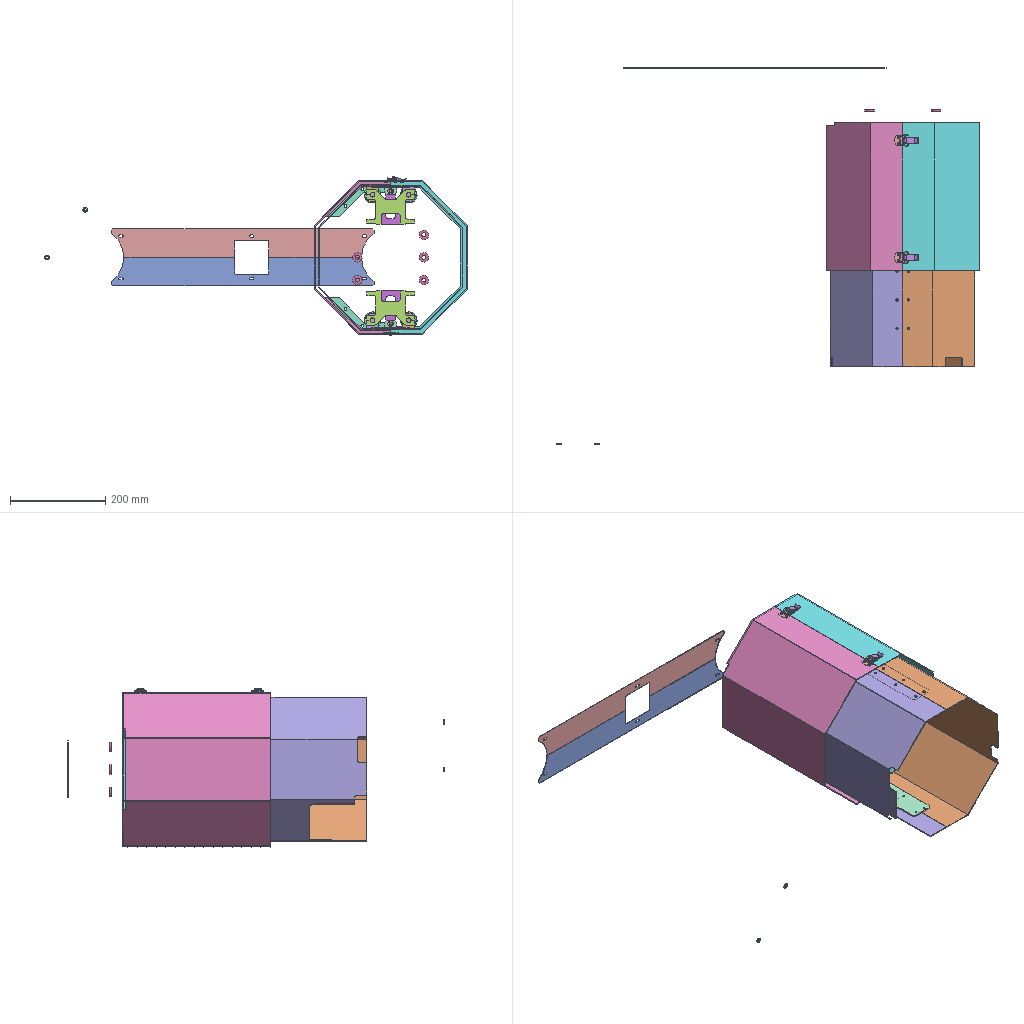Assembly | SolidWorks | 34 different items | 71 placed | box 888 x 792 x 334 mm
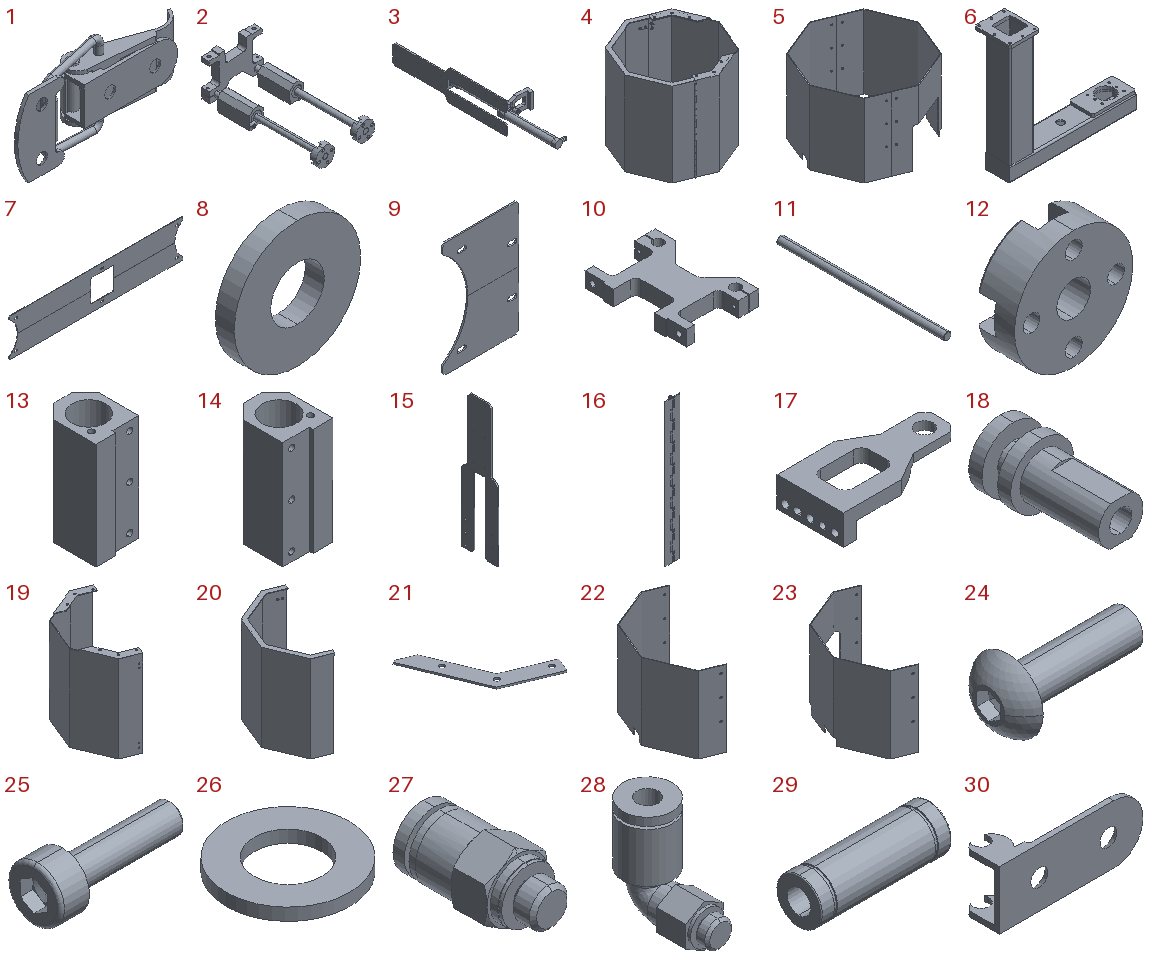Parts list (item | name | quantity | parent item | size | volume | features):
1 | (subassembly) | x2 | in 4 | 49.218 x 9 x 24.478 mm | 2029 mm3 | -
2 | (subassembly) | x1 | - | 110.938 x 220 x 82.039 mm | 184270 mm3 | -
3 | (subassembly) | x2 | - | 80 x 426 x 80 mm | 107986 mm3 | -
4 | (subassembly) | x1 | - | 348.53 x 348.53 x 310 mm | 714229 mm3 | features CompositeCurve 4
5 | (subassembly) | x1 | - | 329.047 x 329.047 x 220 mm | 403476 mm3 | -
6 | - | x1 | - | 855 x 230 x 810 mm | 8405482 mm3 | features ICE 7, HoleWzd 4, Cut 3, Fillet 3, Chamfer 2, CirPattern 2, WeldMemberFeat 2, LPattern 1, WeldCornerFeat 1, WeldmentFeature 1
7 | - | x1 | - | 552 x 1.5 x 120 mm | 85515 mm3 | features ICE 5, Chamfer 2, Extrusion 1, MirrorPattern 1
8 | - | x6 | - | 20 x 3 x 20 mm | 772.243 mm3 | features Extrusion 1
9 | - | x1 | - | 80 x 1.5 x 120 mm | 11312 mm3 | features ICE 6, Chamfer 4, Extrusion 1
10 | - | x2 | in 2 | 71.8 x 102 x 15 mm | 54692 mm3 | features ICE 12, 3DProfileFeature 2, Chamfer 2, HoleWzd 2, Extrusion 1, Fillet 1
11 | - | x4 | in 2 | 10 x 220 x 10 mm | 17254 mm3 | features Chamfer 1, Extrusion 1, ICE 1
12 | - | x4 | in 2 | 35 x 12 x 35 mm | 8080 mm3 | features ICE 2, Chamfer 1, CirPattern 1, Cut 1, Extrusion 1, HoleWzd 1, RefAxis 1
13 | - | x2 | in 2 | 26 x 32 x 60 mm | 27463 mm3 | features ICE 3, HoleWzd 2, 3DProfileFeature 1, Chamfer 1, Extrusion 1
14 | - | x2 | in 2 | 26 x 32 x 60 mm | 27463 mm3 | features ICE 3, 3DProfileFeature 2, HoleWzd 2, Chamfer 1, Extrusion 1
15 | - | x2 | in 3 | 18 x 80 x 300 mm | 47731 mm3 | features ICE 7, Chamfer 4, LPattern 2, 3DProfileFeature 1, Extrusion 1, Fillet 1, HoleWzd 1
16 | - | x1 | in 4 | 32 x 6.5 x 300 mm | 21876 mm3 | features BaseBody 3
17 | - | x2 | in 3 | 79 x 40 x 18 mm | 15138 mm3 | features ICE 6, Chamfer 2, Extrusion 1, HoleWzd 1
18 | - | x2 | in 3 | 12 x 23 x 12 mm | 1299 mm3 | features ICE 5, 3DProfileFeature 1, Extrusion 1, HoleWzd 1
19 | - | x1 | in 4 | 235.877 x 323.01 x 310 mm | 338319 mm3 | features ICE 5, Cut 1, Extrusion 1, HoleWzd 1, RefAxis 1, Shell 1
20 | - | x1 | in 4 | 235.877 x 323.01 x 310 mm | 339899 mm3 | features ICE 4, Extrusion 1, HoleWzd 1, RefAxis 1, Shell 1
21 | - | x2 | in 4 | 102.016 x 112.94 x 2 mm | 5038 mm3 | features ICE 6, Cut 1, Extrusion 1, Shell 1
22 | - | x1 | in 5 | 222.691 x 304.953 x 220 mm | 216770 mm3 | features Cut 2, Fillet 2, ICE 2, Extrusion 1, RefAxis 1, Shell 1
23 | - | x1 | in 5 | 222.691 x 304.953 x 220 mm | 186706 mm3 | features ICE 6, Fillet 3, Cut 2, Extrusion 1, RefAxis 1, Shell 1
24 | - | x4 | in 2 | 23.3 x 12 x 12 mm | 775.96 mm3 | features Cut 2, RevCut 2, Boss 1, Extrusion 1, Fillet 1, LPattern 1
25 | - | x4 | in 2 | 7.6 x 3 x 3 mm | 21.652 mm3 | features Fillet 2, RevCut 2, Boss 1, Chamfer 1, Cut 1, Extrusion 1, LPattern 1
26 | - | x2 | - | 10 x 10 x 1 mm | 54.782 mm3 | features Extrusion 1
27 | - | x2 | in 3 | 8 x 17 x 9.238 mm | 564.577 mm3 | features BaseBody 1
28 | - | x2 | in 3 | 9.3 x 18.35 x 19.641 mm | 1123 mm3 | features BaseBody 1
29 | - | x4 | in 2 | 55 x 19 x 19 mm | 11195 mm3 | features BaseBody 1
30 | - | x2 | in 1 | 27 x 6.688 x 11 mm | 310.781 mm3 | features RefAxis 3, ICE 2, RevCut 2, 3DProfileFeature 1, Extrusion 1
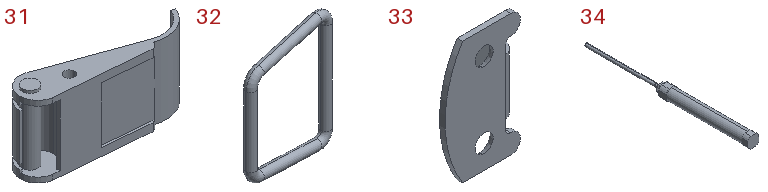31 | - | x2 | in 1 | 30 x 8.531 x 15 mm | 1203 mm3 | features ICE 6, RefAxis 6, 3DProfileFeature 2, Extrusion 1
32 | - | x2 | in 1 | 19.288 x 3.878 x 24.478 mm | 228.547 mm3 | features RefAxis 6, Revolution 4, ICE 3, 3DProfileFeature 2, Extrusion 1
33 | - | x2 | in 1 | 13.5 x 6.5 x 22 mm | 286.659 mm3 | features RefAxis 3, ICE 2, RevCut 2, 3DProfileFeature 1, Extrusion 1
34 | - | x2 | in 3 | 18.3 x 275 x 18.3 mm | 42130 mm3 | features ICE 6, Chamfer 3, Extrusion 1, HoleWzd 1
Mates (type | each side: item.copy, entity, surface, feature):
In the top assembly
Coincident | 14.1 face plane Boss-Extrude1 | 15.1 face plane Boss-Extrude1
Concentric | 14.1 face cylinder M4 Tapped Hole1 | 15.1 face cylinder Cut-Extrude6
Concentric | 14.1 face cylinder M4 Tapped Hole1 | 15.1 face cylinder LPattern2
Concentric | 15.2 face cylinder LPattern1 | 23.1 face cylinder Cut-Extrude2 | 2 times
Coincident | 15.2 face plane Boss-Extrude1 | 23.1 face plane Shell1
Coincident | 7.1 face plane Boss-Extrude1 | 6.1 face plane Structural Member2
Parallel | 7.1 face plane Boss-Extrude1 | 6.1 face plane Structural Member2
Concentric | 7.1 face cylinder Cut-Extrude10 | 6.1 face cylinder Cut-Extrude3
Coincident | 7.1 face plane Boss-Extrude1 | 9.1 face plane Boss-Extrude1
Coincident | 6.1 face plane Structural Member2 | 8.1 face plane Boss-Extrude1
Concentric | 8.1 face cylinder Boss-Extrude1 | 6.1 face cylinder Cut-Extrude2
Coincident | 6.1 face plane Structural Member2 | 9.1 face plane Boss-Extrude1
Concentric | 6.1 face cylinder Cut-Extrude3 | 9.1 face cylinder Cut-Extrude10
Concentric | 6.1 face cylinder Ø12.0 (12) Diameter Hole1 | 26.1 face cylinder Base-Extrude
Coincident | 6.1 face plane Boss-Extrude3 | 26.1 face plane Base-Extrude
Coincident | 6.1 face plane Boss-Extrude3 | 26.2 face plane Base-Extrude
Concentric | 6.1 face cylinder Ø12.0 (12) Diameter Hole1 | 26.2 face cylinder Base-Extrude
Concentric | 11.1 face cylinder Boss-Extrude1 | 10.1 face cylinder Cut-Extrude2
Concentric | 10.1 face cylinder Boss-Extrude3 | 11.2 face cylinder Boss-Extrude1
Coincident | 10.1 face plane Boss-Extrude1 | 11.2 face plane Boss-Extrude1
Coincident | 10.1 face plane Boss-Extrude1 | 11.1 face plane Boss-Extrude1
DistanceDim | 14.2 face plane Boss-Extrude1 | 10.1 face plane Boss-Extrude1
Concentric | 10.1 face cylinder Cut-Extrude8 | 25.1 face cylinder BaseBody
Coincident | 10.1 face plane Boss-Extrude3 | 25.1 face plane BaseHead
Concentric | 10.1 face cylinder Cut-Extrude8 | 25.2 face cylinder BaseBody
Coincident | 10.1 face plane Boss-Extrude1 | 25.2 face plane BaseHead
Concentric | 11.1 face cylinder Boss-Extrude1 | 12.1 face cylinder Boss-Extrude1
Concentric | 11.1 face cylinder Boss-Extrude1 | 29.1 face cylinder Input1
Concentric | 11.2 face cylinder Boss-Extrude1 | 12.2 face cylinder Boss-Extrude1
Coincident | 11.2 face plane Boss-Extrude1 | 12.2 face plane Boss-Extrude1
Concentric | 11.2 face cylinder Boss-Extrude1 | 14.2 face cylinder Boss-Extrude2
Concentric | 11.2 face cylinder Boss-Extrude1 | 29.2 face cylinder Input1
Coincident | 12.1 face plane Boss-Extrude1 | 12.2 face plane Boss-Extrude1
Coincident | 13.1 face plane Boss-Extrude1 | 14.2 face plane Boss-Extrude1
Parallel | 13.1 face plane Boss-Extrude1 | 14.2 face plane Boss-Extrude1
Coincident | 13.1 face plane Boss-Extrude3 | 14.2 face plane Boss-Extrude3
Concentric | 13.1 face cylinder M4 Tapped Hole3 | 24.1 face cylinder BaseBody
Coincident | 13.1 face plane Boss-Extrude1 | 24.1 face plane BaseHead
Concentric | 13.1 face cylinder Boss-Extrude1 | 29.1 face cylinder Input1
Coincident | 13.1 face plane Boss-Extrude2 | 29.1 face plane Input1
Concentric | 14.2 face cylinder M4 Tapped Hole2 | 24.2 face cylinder BaseBody
Coincident | 14.2 face plane Boss-Extrude1 | 24.2 face plane BaseHead
Concentric | 14.2 face cylinder Boss-Extrude1 | 29.2 face cylinder Input1
Coincident | 14.2 face plane Boss-Extrude2 | 29.2 face plane Input1
Concentric | 13.1 face cylinder M4 Tapped Hole1 | 15.2 face cylinder Cut-Extrude6
Concentric | 13.1 face cylinder M4 Tapped Hole1 | 15.2 face cylinder LPattern2
Coincident | 13.1 face plane Boss-Extrude1 | 15.2 face plane Boss-Extrude1
In subassembly 5
Coincident | 22.1 face plane Cut-Extrude1 | 23.2 face plane Cut-Extrude1
Coincident | 22.1 face plane Boss-Extrude1 | 23.2 face plane Boss-Extrude1
In subassembly 4
Coincident | 19.1 face plane Boss-Extrude1 | 20.1 face plane Boss-Extrude1 | 2 times
Concentric | 19.1 face cylinder M3 Tapped Hole1 | 33.1 edge | 2 times
Coincident | 19.1 face plane Boss-Extrude1 | 33.1 face plane Boss-Extrude1
Concentric | 19.1 face cylinder M3 Tapped Hole1 | 33.2 edge | 2 times
Coincident | 19.1 face plane Boss-Extrude1 | 33.2 face plane Boss-Extrude1
Coincident | 19.1 face plane Cut-Extrude2 | 20.1 face plane Cut-Extrude2
Coincident | 20.1 face plane Shell1 | 16.1 face plane 2-1-solid1
Coincident | 20.1 face plane Boss-Extrude1 | 16.1 face plane 1-1-solid1
DistanceDim | 16.1 face plane 2-1-solid1 | 20.1 face plane Cut-Extrude3
Coincident | 19.1 face plane Shell1 | 21.1 face plane Boss-Extrude1
Concentric | 19.1 face cylinder Cut-Extrude4 | 21.1 face cylinder Cut-Extrude4 | 2 times
Coincident | 19.1 face plane Shell1 | 21.2 face plane Shell1
Concentric | 19.1 face cylinder Cut-Extrude4 | 21.2 face cylinder Cut-Extrude4 | 2 times
In subassembly 1
Coincident | 30.1 plane | 31.1 plane
Coincident | 30.1 axis | 31.1 axis
Coincident | 31.1 plane | 32.1 plane
Coincident | 31.1 axis | 32.1 axis
Coincident | 32.1 plane | 33.3 plane
Coincident | 32.1 axis | 33.3 axis
In subassembly 2
Concentric | 11.1 face cylinder Boss-Extrude1 | 12.1 face cylinder Boss-Extrude1
Concentric | 11.1 face cylinder Boss-Extrude1 | 10.1 face cylinder Cut-Extrude2
Concentric | 10.1 face cylinder Boss-Extrude3 | 11.2 face cylinder Boss-Extrude1
Coincident | 10.1 face plane Boss-Extrude1 | 11.2 face plane Boss-Extrude1
Concentric | 11.2 face cylinder Boss-Extrude1 | 12.2 face cylinder Boss-Extrude1
Coincident | 11.2 face plane Boss-Extrude1 | 12.2 face plane Boss-Extrude1
Concentric | 11.2 face cylinder Boss-Extrude1 | 14.3 face cylinder Boss-Extrude2
Coincident | 13.1 face plane Boss-Extrude1 | 14.3 face plane Boss-Extrude1
Parallel | 13.1 face plane Boss-Extrude1 | 14.3 face plane Boss-Extrude1
Coincident | 10.1 face plane Boss-Extrude1 | 11.1 face plane Boss-Extrude1
Coincident | 12.1 face plane Boss-Extrude1 | 12.2 face plane Boss-Extrude1
Coincident | 13.1 face plane Boss-Extrude3 | 14.3 face plane Boss-Extrude3
DistanceDim | 14.3 face plane Boss-Extrude1 | 10.1 face plane Boss-Extrude1
Concentric | 14.3 face cylinder M4 Tapped Hole2 | 24.1 face cylinder BaseBody
Coincident | 14.3 face plane Boss-Extrude1 | 24.1 face plane BaseHead
Concentric | 13.1 face cylinder M4 Tapped Hole3 | 24.3 face cylinder BaseBody
Coincident | 13.1 face plane Boss-Extrude1 | 24.3 face plane BaseHead
Concentric | 10.1 face cylinder Cut-Extrude8 | 25.2 face cylinder BaseBody
Coincident | 10.1 face plane Boss-Extrude3 | 25.2 face plane BaseHead
Concentric | 10.1 face cylinder Cut-Extrude8 | 25.3 face cylinder BaseBody
Coincident | 10.1 face plane Boss-Extrude1 | 25.3 face plane BaseHead
Concentric | 11.1 face cylinder Boss-Extrude1 | 29.3 face cylinder Input1
Concentric | 11.2 face cylinder Boss-Extrude1 | 29.1 face cylinder Input1
Concentric | 14.3 face cylinder Boss-Extrude1 | 29.1 face cylinder Input1
Concentric | 13.1 face cylinder Boss-Extrude1 | 29.3 face cylinder Input1
Coincident | 13.1 face plane Boss-Extrude2 | 29.3 face plane Input1
Coincident | 14.3 face plane Boss-Extrude2 | 29.1 face plane Input1
In subassembly 3
Coincident | 34.1 face plane Boss-Extrude1 | 17.1 face plane Cut-Extrude6
DistanceDim | 17.1 face plane Boss-Extrude1 | 15.3 face plane Boss-Extrude1
Concentric | 34.1 face cylinder Boss-Extrude4 | 17.1 face cylinder Cut-Extrude2
Parallel | 17.1 face plane Boss-Extrude1 | 34.1 face plane Boss-Extrude1
DistanceDim | 15.3 face plane Boss-Extrude1 | 17.1 face plane Boss-Extrude1
Concentric | 34.1 face cylinder Boss-Extrude6 | 18.1 face cylinder Boss-Extrude4
Coincident | 15.3 face plane Boss-Extrude1 | 18.1 face plane Boss-Extrude2
Width | 17.1 face plane Boss-Extrude1 | 17.1 face plane Boss-Extrude1 | 15.3 face plane Boss-Extrude1 | 15.3 face plane Boss-Extrude1
Coincident | 34.1 face plane Boss-Extrude1 | 28.1 face plane Input1
Concentric | 34.1 face cylinder M5 Tapped Hole1 | 28.1 face cylinder Input1
Concentric | 34.1 face cylinder M5 Tapped Hole1 | 27.1 face cylinder Input1
Coincident | 34.1 face plane Boss-Extrude3 | 27.1 face plane Input1